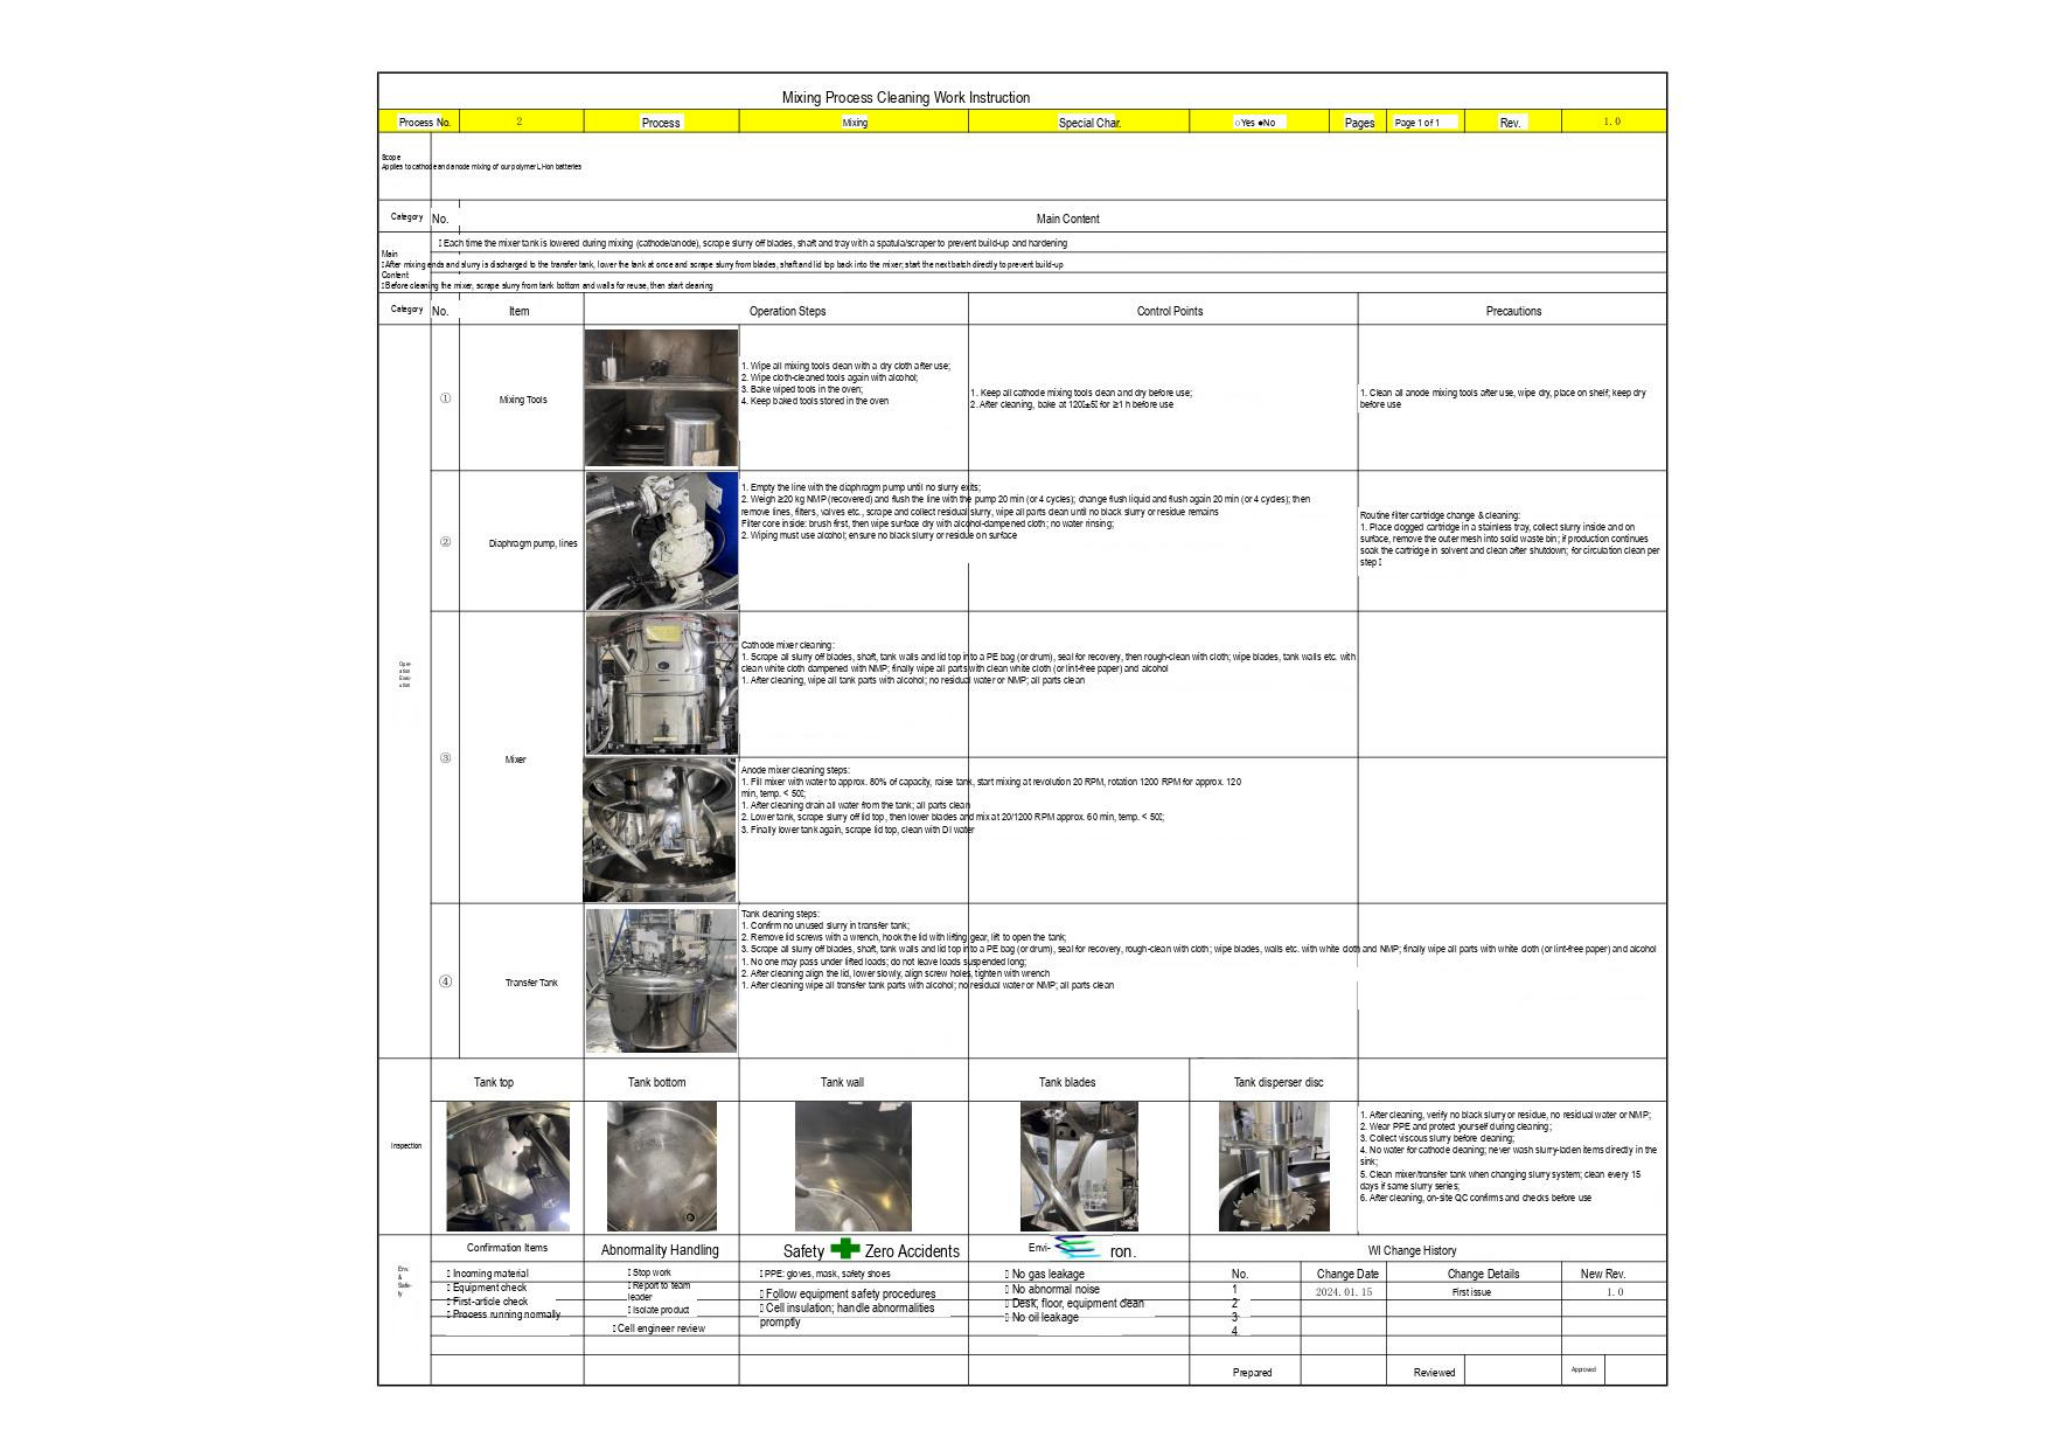Mixing Process Cleaning Work Instruction

| Process No. | 2 | Process | Mixing | Special Char. | ○Yes ●No | Pages | Page 1 of 1 | Rev. | 1.0 |
|---|---|---|---|---|---|---|---|---|---|

Scope
Applies to cathode and anode mixing of our polymer Li-ion batteries

| Category | No. | Main Content |
|---|---|---|
| Main Content | | Each time the mixer tank is lowered during mixing (cathode/anode), scrape slurry off blades, shaft and tray with a spatula/scraper to prevent build-up and hardening |
| | | After mixing ends and slurry is discharged to the transfer tank, lower the tank at once and scrape slurry from blades, shaft and lid top back into the mixer; start the next batch directly to prevent build-up |
| | | Before cleaning the mixer, scrape slurry from tank bottom and walls for reuse, then start cleaning |

| Category | No. | Item | Operation Steps | Control Points | Precautions |
|---|---|---|---|---|---|
| Operation Description | ① | Mixing Tools | 1. Wipe all mixing tools clean with a dry cloth after use;<br>2. Wipe cloth-cleaned tools again with alcohol;<br>3. Bake wiped tools in the oven;<br>4. Keep baked tools stored in the oven | 1. Keep all cathode mixing tools clean and dry before use;<br>2. After cleaning, bake at 120±5 for ≥1 h before use | 1. Clean all anode mixing tools after use, wipe dry, place on shelf, keep dry before use |
| | ② | Diaphragm pump, lines | 1. Empty the line with the diaphragm pump until no slurry exits;<br>2. Weigh ≥20 kg NMP (recovered) and flush the line with the pump 20 min (or 4 cycles); change flush liquid and flush again 20 min (or 4 cycles); then remove lines, filters, valves etc., scrape and collect residual slurry, wipe all parts clean until no black slurry or residue remains<br>Filter core inside: brush first, then wipe surface dry with alcohol-dampened cloth; no water rinsing;<br>2. Wiping must use alcohol; ensure no black slurry or residue on surface | | Routine filter cartridge change & cleaning:<br>1. Place clogged cartridge in a stainless tray, collect slurry inside and on surface, remove the outer mesh into solid waste bin; if production continues soak the cartridge in solvent and clean after shutdown; for circulation clean per step |
| | ③ | Mixer | Cathode mixer cleaning:<br>1. Scrape all slurry off blades, shaft, tank walls and lid top into a PE bag (or drum), seal for recovery, then rough-clean with cloth; wipe blades, tank walls etc. with clean white cloth dampened with NMP; finally wipe all parts with clean white cloth (or lint-free paper) and alcohol<br>1. After cleaning, wipe all tank parts with alcohol; no residual water or NMP; all parts clean | | |
| | | | Anode mixer cleaning steps:<br>1. Fill mixer with water to approx. 80% of capacity, raise tank, start mixing at revolution 20 RPM, rotation 1200 RPM for approx. 120 min, temp. < 50;<br>1. After cleaning drain all water from the tank; all parts clean<br>2. Lower tank, scrape slurry off lid top, then lower blades and mix at 20/1200 RPM approx. 60 min, temp. < 50;<br>3. Finally lower tank again, scrape lid top, clean with DI water | | |
| | ④ | Transfer Tank | Tank cleaning steps:<br>1. Confirm no unused slurry in transfer tank;<br>2. Remove lid screws with a wrench, hook the lid with lifting gear, lift to open the tank;<br>3. Scrape all slurry off blades, shaft, tank walls and lid top into a PE bag (or drum), seal for recovery, rough-clean with cloth; wipe blades, walls etc. with white cloth and NMP; finally wipe all parts with white cloth (or lint-free paper) and alcohol<br>1. No one may pass under lifted loads; do not leave loads suspended long;<br>2. After cleaning align the lid, lower slowly, align screw holes, tighten with wrench<br>1. After cleaning wipe all transfer tank parts with alcohol; no residual water or NMP; all parts clean | | |

| Inspection | Tank top | Tank bottom | Tank wall | Tank blades | Tank disperser disc | |
|---|---|---|---|---|---|---|
| | | | | | | 1. After cleaning, verify no black slurry or residue, no residual water or NMP;<br>2. Wear PPE and protect yourself during cleaning;<br>3. Collect viscous slurry before cleaning;<br>4. No water for cathode cleaning; never wash slurry-laden items directly in the sink;<br>5. Clean mixer/transfer tank when changing slurry system; clean every 15 days if same slurry series;<br>6. After cleaning, on-site QC confirms and checks before use |

| Env. & Safety | Confirmation Items | Abnormality Handling | Safety Zero Accidents | Envi-ron. |
|---|---|---|---|---|
| | Incoming material<br>Equipment check<br>First-article check<br>Process running normally | Stop work<br>Report to team leader<br>Isolate product<br>Cell engineer review | PPE: gloves, mask, safety shoes<br>Follow equipment safety procedures<br>Cell insulation; handle abnormalities promptly | No gas leakage<br>No abnormal noise<br>Desk, floor, equipment clean<br>No oil leakage |

WI Change History

| No. | Change Date | Change Details | New Rev. |
|---|---|---|---|
| 1 | 2024.01.15 | First issue | 1.0 |
| 2 | | | |
| 3 | | | |
| 4 | | | |

| Prepared | | Reviewed | | Approved | |
|---|---|---|---|---|---|